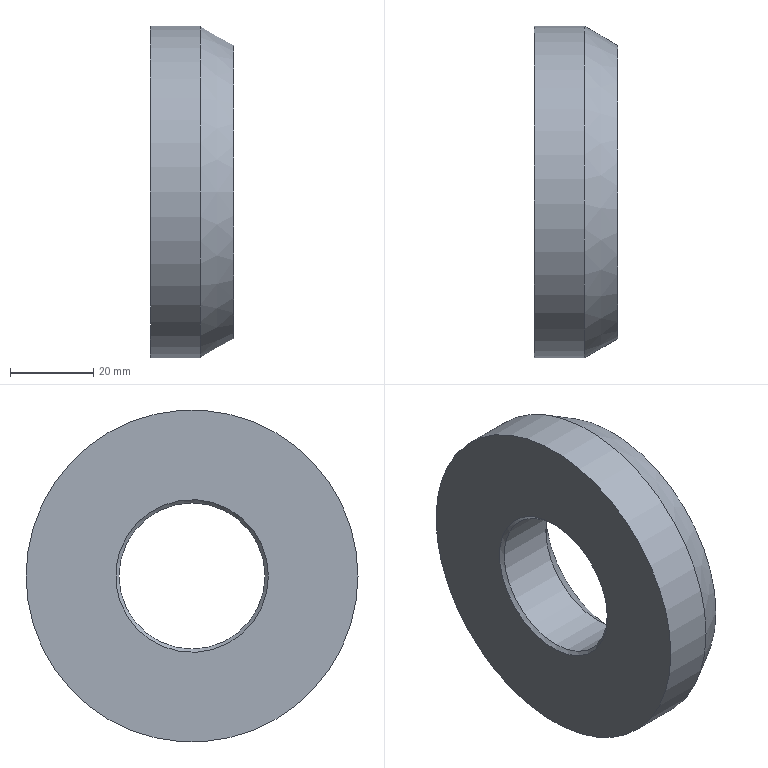Part | NX | features solid 2 | 1 solid | 7 faces | box 20 x 80 x 80 mm | volume 75054 mm3 | cone 3 | cylinder 2 | plane 2 | commonest cylinder face diameters 35.2 x1 80 x1
STEP:
#1=CARTESIAN_POINT('',(-1833.2,-1227.6,-480.));
#2=VERTEX_POINT('',#1);
#3=CARTESIAN_POINT('',(-1833.2,-1210.,-480.));
#4=DIRECTION('',(-1.,0.,0.));
#5=DIRECTION('',(0.,-1.,0.));
#6=AXIS2_PLACEMENT_3D('',#3,#4,#5);
#7=CIRCLE('',#6,17.6);
#8=EDGE_CURVE('',#2,#2,#7,.T.);
#9=ORIENTED_EDGE('',*,*,#8,.T.);
#10=EDGE_LOOP('',(#9));
#11=FACE_BOUND('',#10,.T.);
#12=CARTESIAN_POINT('',(-1819.,-1227.6,-480.));
#13=VERTEX_POINT('',#12);
#14=CARTESIAN_POINT('',(-1819.,-1210.,-480.));
#15=DIRECTION('',(-1.,0.,0.));
#16=DIRECTION('',(0.,-1.,0.));
#17=AXIS2_PLACEMENT_3D('',#14,#15,#16);
#18=CIRCLE('',#17,17.6);
#19=EDGE_CURVE('',#13,#13,#18,.F.);
#20=ORIENTED_EDGE('',*,*,#19,.T.);
#21=EDGE_LOOP('',(#20));
#22=FACE_BOUND('',#21,.T.);
#23=CARTESIAN_POINT('',(-1814.,-1210.,-480.));
#24=DIRECTION('',(-1.,0.,0.));
#25=DIRECTION('',(0.,-1.,0.));
#26=AXIS2_PLACEMENT_3D('',#23,#24,#25);
#27=CYLINDRICAL_SURFACE('',#26,17.6);
#28=ADVANCED_FACE('',(#11,#22),#27,.F.);
#29=CARTESIAN_POINT('',(-1822.,-1250.,-480.));
#30=VERTEX_POINT('',#29);
#31=CARTESIAN_POINT('',(-1822.,-1210.,-480.));
#32=DIRECTION('',(-1.,0.,0.));
#33=DIRECTION('',(0.,-1.,0.));
#34=AXIS2_PLACEMENT_3D('',#31,#32,#33);
#35=CIRCLE('',#34,40.);
#36=EDGE_CURVE('',#30,#30,#35,.T.);
#37=ORIENTED_EDGE('',*,*,#36,.T.);
#38=EDGE_LOOP('',(#37));
#39=FACE_BOUND('',#38,.T.);
#40=CARTESIAN_POINT('',(-1834.,-1250.,-480.));
#41=VERTEX_POINT('',#40);
#42=CARTESIAN_POINT('',(-1834.,-1210.,-480.));
#43=DIRECTION('',(-1.,0.,0.));
#44=DIRECTION('',(0.,-1.,0.));
#45=AXIS2_PLACEMENT_3D('',#42,#43,#44);
#46=CIRCLE('',#45,40.);
#47=EDGE_CURVE('',#41,#41,#46,.T.);
#48=ORIENTED_EDGE('',*,*,#47,.F.);
#49=EDGE_LOOP('',(#48));
#50=FACE_BOUND('',#49,.T.);
#51=CARTESIAN_POINT('',(-1814.,-1210.,-480.));
#52=DIRECTION('',(-1.,0.,0.));
#53=DIRECTION('',(0.,-1.,0.));
#54=AXIS2_PLACEMENT_3D('',#51,#52,#53);
#55=CYLINDRICAL_SURFACE('',#54,40.);
#56=ADVANCED_FACE('',(#39,#50),#55,.T.);
#57=CARTESIAN_POINT('',(-1814.,-1232.6,-480.));
#58=VERTEX_POINT('',#57);
#59=CARTESIAN_POINT('',(-1814.,-1210.,-480.));
#60=DIRECTION('',(-1.,0.,0.));
#61=DIRECTION('',(0.,-1.,0.));
#62=AXIS2_PLACEMENT_3D('',#59,#60,#61);
#63=CIRCLE('',#62,22.6);
#64=EDGE_CURVE('',#58,#58,#63,.T.);
#65=ORIENTED_EDGE('',*,*,#64,.T.);
#66=EDGE_LOOP('',(#65));
#67=FACE_BOUND('',#66,.T.);
#68=CARTESIAN_POINT('',(-1814.,-1245.381,-480.));
#69=VERTEX_POINT('',#68);
#70=CARTESIAN_POINT('',(-1814.,-1210.,-480.));
#71=DIRECTION('',(-1.,0.,0.));
#72=DIRECTION('',(0.,-1.,0.));
#73=AXIS2_PLACEMENT_3D('',#70,#71,#72);
#74=CIRCLE('',#73,35.381);
#75=EDGE_CURVE('',#69,#69,#74,.F.);
#76=ORIENTED_EDGE('',*,*,#75,.T.);
#77=EDGE_LOOP('',(#76));
#78=FACE_BOUND('',#77,.T.);
#79=CARTESIAN_POINT('',(-1814.,-1210.,-480.));
#80=DIRECTION('',(-1.,0.,0.));
#81=DIRECTION('',(0.,-1.,0.));
#82=AXIS2_PLACEMENT_3D('',#79,#80,#81);
#83=PLANE('',#82);
#84=ADVANCED_FACE('',(#67,#78),#83,.F.);
#85=CARTESIAN_POINT('',(-1834.,-1228.4,-480.));
#86=VERTEX_POINT('',#85);
#87=CARTESIAN_POINT('',(-1834.,-1210.,-480.));
#88=DIRECTION('',(-1.,0.,0.));
#89=DIRECTION('',(0.,-1.,0.));
#90=AXIS2_PLACEMENT_3D('',#87,#88,#89);
#91=CIRCLE('',#90,18.4);
#92=EDGE_CURVE('',#86,#86,#91,.F.);
#93=ORIENTED_EDGE('',*,*,#92,.T.);
#94=EDGE_LOOP('',(#93));
#95=FACE_BOUND('',#94,.T.);
#96=ORIENTED_EDGE('',*,*,#47,.T.);
#97=EDGE_LOOP('',(#96));
#98=FACE_BOUND('',#97,.T.);
#99=CARTESIAN_POINT('',(-1834.,-1210.,-480.));
#100=DIRECTION('',(-1.,0.,0.));
#101=DIRECTION('',(0.,-1.,0.));
#102=AXIS2_PLACEMENT_3D('',#99,#100,#101);
#103=PLANE('',#102);
#104=ADVANCED_FACE('',(#95,#98),#103,.T.);
#105=ORIENTED_EDGE('',*,*,#75,.F.);
#106=EDGE_LOOP('',(#105));
#107=FACE_BOUND('',#106,.T.);
#108=ORIENTED_EDGE('',*,*,#36,.F.);
#109=EDGE_LOOP('',(#108));
#110=FACE_BOUND('',#109,.T.);
#111=CARTESIAN_POINT('',(-1822.,-1210.,-480.));
#112=DIRECTION('',(-1.,0.,0.));
#113=DIRECTION('',(0.,-1.,0.));
#114=AXIS2_PLACEMENT_3D('',#111,#112,#113);
#115=CONICAL_SURFACE('',#114,40.,0.5236);
#116=ADVANCED_FACE('',(#107,#110),#115,.T.);
#117=ORIENTED_EDGE('',*,*,#19,.F.);
#118=EDGE_LOOP('',(#117));
#119=FACE_BOUND('',#118,.T.);
#120=ORIENTED_EDGE('',*,*,#64,.F.);
#121=EDGE_LOOP('',(#120));
#122=FACE_BOUND('',#121,.T.);
#123=CARTESIAN_POINT('',(-1814.,-1210.,-480.));
#124=DIRECTION('',(1.,0.,0.));
#125=DIRECTION('',(0.,1.,0.));
#126=AXIS2_PLACEMENT_3D('',#123,#124,#125);
#127=CONICAL_SURFACE('',#126,22.6,0.7854);
#128=ADVANCED_FACE('',(#119,#122),#127,.F.);
#129=ORIENTED_EDGE('',*,*,#92,.F.);
#130=EDGE_LOOP('',(#129));
#131=FACE_BOUND('',#130,.T.);
#132=ORIENTED_EDGE('',*,*,#8,.F.);
#133=EDGE_LOOP('',(#132));
#134=FACE_BOUND('',#133,.T.);
#135=CARTESIAN_POINT('',(-1833.2,-1210.,-480.));
#136=DIRECTION('',(-1.,0.,0.));
#137=DIRECTION('',(0.,-1.,0.));
#138=AXIS2_PLACEMENT_3D('',#135,#136,#137);
#139=CONICAL_SURFACE('',#138,17.6,0.7854);
#140=ADVANCED_FACE('',(#131,#134),#139,.F.);
#141=CLOSED_SHELL('',(#28,#56,#84,#104,#116,#128,#140));
#142=MANIFOLD_SOLID_BREP('',#141);
#143=(LENGTH_UNIT()NAMED_UNIT(*)SI_UNIT(.MILLI.,.METRE.));
#144=UNCERTAINTY_MEASURE_WITH_UNIT(LENGTH_MEASURE(0.00001),#143,'','');
#145=(NAMED_UNIT(*)PLANE_ANGLE_UNIT()SI_UNIT($,.RADIAN.));
#146=(NAMED_UNIT(*)SI_UNIT($,.STERADIAN.)SOLID_ANGLE_UNIT());
#147=(GEOMETRIC_REPRESENTATION_CONTEXT(3)GLOBAL_UNCERTAINTY_ASSIGNED_CONTEXT((#144))GLOBAL_UNIT_ASSIGNED_CONTEXT((#143,#145,#146))REPRESENTATION_CONTEXT('',''));
#148=ADVANCED_BREP_SHAPE_REPRESENTATION('',(#142),#147);